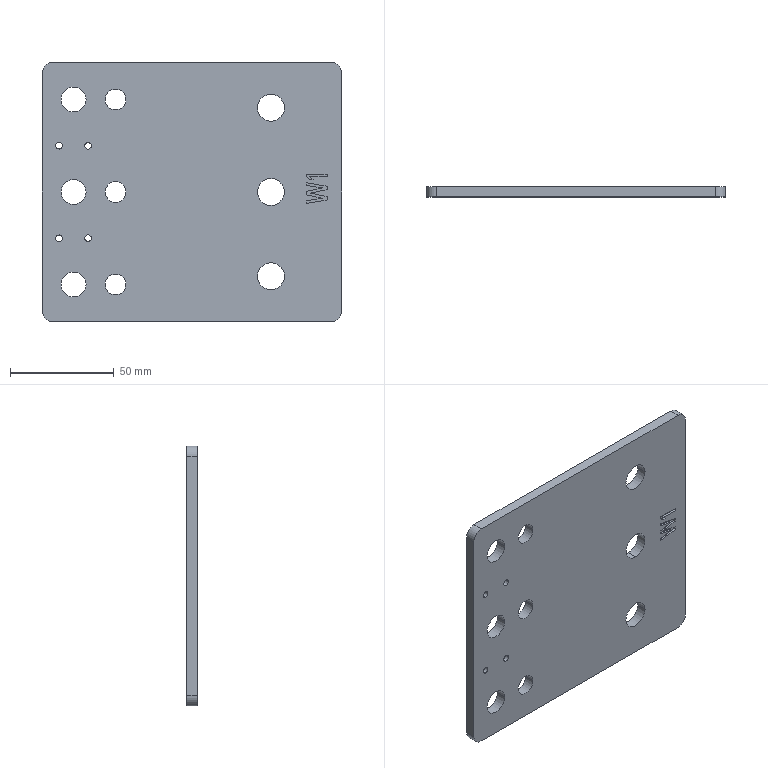Part | STEP file | SOLID | 1 solid | 58 faces | box 144 x 5 x 125 mm | volume 84805 mm3 | cylinder 30 | plane 28 | commonest cylinder face diameters 10 x10 3.2 x8 12 x6 13 x6